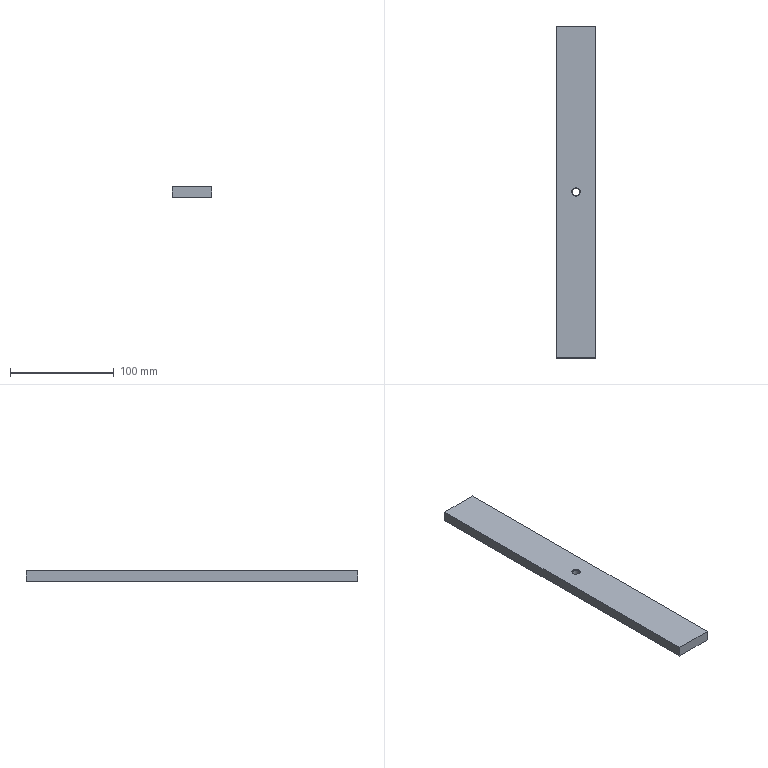Part | STEP file | A14-040 | 1 solid | 10 faces | box 38 x 320 x 10 mm | volume 121232 mm3 | plane 6 | cone 2 | cylinder 2 | commonest cylinder face diameters 6.8 x2
STEP:
#1=CARTESIAN_POINT('',(0.,0.,0.));
#2=DIRECTION('',(0.,0.,1.));
#3=DIRECTION('',(1.,0.,0.));
#4=AXIS2_PLACEMENT_3D('',#1,#2,#3);
#5=CARTESIAN_POINT('',(3.4,0.,4.375));
#6=VERTEX_POINT('',#5);
#7=CARTESIAN_POINT('',(4.025,0.,5.));
#8=VERTEX_POINT('',#7);
#9=CARTESIAN_POINT('',(4.025,0.,5.));
#10=DIRECTION('',(0.7071,0.,0.7071));
#11=VECTOR('',#10,1.);
#12=LINE('',#9,#11);
#13=CARTESIAN_POINT('',(0.,0.,5.));
#14=DIRECTION('',(0.,0.,1.));
#15=DIRECTION('',(1.,0.,0.));
#16=AXIS2_PLACEMENT_3D('',#13,#14,#15);
#17=CONICAL_SURFACE('',#16,4.025,0.7854);
#18=CARTESIAN_POINT('',(6.283,0.));
#19=DIRECTION('',(0.,1.));
#20=VECTOR('',#19,1.);
#21=LINE('',#18,#20);
#22=(GEOMETRIC_REPRESENTATION_CONTEXT(2)PARAMETRIC_REPRESENTATION_CONTEXT()REPRESENTATION_CONTEXT('',''));
#23=DEFINITIONAL_REPRESENTATION('',(#21),#22);
#24=PCURVE('',#17,#23);
#25=CARTESIAN_POINT('',(0.,0.,5.));
#26=DIRECTION('',(0.,0.,1.));
#27=DIRECTION('',(1.,0.,0.));
#28=AXIS2_PLACEMENT_3D('',#25,#26,#27);
#29=CONICAL_SURFACE('',#28,4.025,0.7854);
#30=CARTESIAN_POINT('',(0.,0.));
#31=DIRECTION('',(0.,1.));
#32=VECTOR('',#31,1.);
#33=LINE('',#30,#32);
#34=(GEOMETRIC_REPRESENTATION_CONTEXT(2)PARAMETRIC_REPRESENTATION_CONTEXT()REPRESENTATION_CONTEXT('',''));
#35=DEFINITIONAL_REPRESENTATION('',(#33),#34);
#36=PCURVE('',#29,#35);
#37=SURFACE_CURVE('',#12,(#24,#36),.PCURVE_S1.);
#38=EDGE_CURVE('',#6,#8,#37,.T.);
#39=ORIENTED_EDGE('',*,*,#38,.T.);
#40=CARTESIAN_POINT('',(-4.025,0.,5.));
#41=VERTEX_POINT('',#40);
#42=CARTESIAN_POINT('',(0.,0.,5.));
#43=DIRECTION('',(0.,0.,1.));
#44=DIRECTION('',(1.,0.,0.));
#45=AXIS2_PLACEMENT_3D('',#42,#43,#44);
#46=CIRCLE('',#45,4.025);
#47=CARTESIAN_POINT('',(0.,0.));
#48=DIRECTION('',(1.,0.));
#49=VECTOR('',#48,1.);
#50=LINE('',#47,#49);
#51=(GEOMETRIC_REPRESENTATION_CONTEXT(2)PARAMETRIC_REPRESENTATION_CONTEXT()REPRESENTATION_CONTEXT('',''));
#52=DEFINITIONAL_REPRESENTATION('',(#50),#51);
#53=PCURVE('',#17,#52);
#54=CARTESIAN_POINT('',(0.,0.,5.));
#55=DIRECTION('',(0.,0.,1.));
#56=DIRECTION('',(1.,0.,0.));
#57=AXIS2_PLACEMENT_3D('',#54,#55,#56);
#58=PLANE('',#57);
#59=CARTESIAN_POINT('',(0.,0.));
#60=DIRECTION('',(1.,0.));
#61=AXIS2_PLACEMENT_2D('',#59,#60);
#62=CIRCLE('',#61,4.025);
#63=(GEOMETRIC_REPRESENTATION_CONTEXT(2)PARAMETRIC_REPRESENTATION_CONTEXT()REPRESENTATION_CONTEXT('',''));
#64=DEFINITIONAL_REPRESENTATION('',(#62),#63);
#65=PCURVE('',#58,#64);
#66=SURFACE_CURVE('',#46,(#53,#65),.PCURVE_S1.);
#67=EDGE_CURVE('',#41,#8,#66,.T.);
#68=ORIENTED_EDGE('',*,*,#67,.F.);
#69=CARTESIAN_POINT('',(-3.4,0.,4.375));
#70=VERTEX_POINT('',#69);
#71=CARTESIAN_POINT('',(-4.025,0.,5.));
#72=DIRECTION('',(-0.7071,0.,0.7071));
#73=VECTOR('',#72,1.);
#74=LINE('',#71,#73);
#75=CARTESIAN_POINT('',(3.142,0.));
#76=DIRECTION('',(0.,1.));
#77=VECTOR('',#76,1.);
#78=LINE('',#75,#77);
#79=(GEOMETRIC_REPRESENTATION_CONTEXT(2)PARAMETRIC_REPRESENTATION_CONTEXT()REPRESENTATION_CONTEXT('',''));
#80=DEFINITIONAL_REPRESENTATION('',(#78),#79);
#81=PCURVE('',#17,#80);
#82=CARTESIAN_POINT('',(3.142,0.));
#83=DIRECTION('',(0.,1.));
#84=VECTOR('',#83,1.);
#85=LINE('',#82,#84);
#86=(GEOMETRIC_REPRESENTATION_CONTEXT(2)PARAMETRIC_REPRESENTATION_CONTEXT()REPRESENTATION_CONTEXT('',''));
#87=DEFINITIONAL_REPRESENTATION('',(#85),#86);
#88=PCURVE('',#29,#87);
#89=SURFACE_CURVE('',#74,(#81,#88),.PCURVE_S1.);
#90=EDGE_CURVE('',#70,#41,#89,.T.);
#91=ORIENTED_EDGE('',*,*,#90,.F.);
#92=CARTESIAN_POINT('',(0.,0.,4.375));
#93=DIRECTION('',(0.,0.,1.));
#94=DIRECTION('',(1.,0.,0.));
#95=AXIS2_PLACEMENT_3D('',#92,#93,#94);
#96=CIRCLE('',#95,3.4);
#97=CARTESIAN_POINT('',(0.,-0.625));
#98=DIRECTION('',(1.,0.));
#99=VECTOR('',#98,1.);
#100=LINE('',#97,#99);
#101=(GEOMETRIC_REPRESENTATION_CONTEXT(2)PARAMETRIC_REPRESENTATION_CONTEXT()REPRESENTATION_CONTEXT('',''));
#102=DEFINITIONAL_REPRESENTATION('',(#100),#101);
#103=PCURVE('',#17,#102);
#104=CARTESIAN_POINT('',(0.,0.,5.));
#105=DIRECTION('',(0.,0.,1.));
#106=DIRECTION('',(1.,0.,0.));
#107=AXIS2_PLACEMENT_3D('',#104,#105,#106);
#108=CYLINDRICAL_SURFACE('',#107,3.4);
#109=CARTESIAN_POINT('',(0.,-0.625));
#110=DIRECTION('',(1.,0.));
#111=VECTOR('',#110,1.);
#112=LINE('',#109,#111);
#113=(GEOMETRIC_REPRESENTATION_CONTEXT(2)PARAMETRIC_REPRESENTATION_CONTEXT()REPRESENTATION_CONTEXT('',''));
#114=DEFINITIONAL_REPRESENTATION('',(#112),#113);
#115=PCURVE('',#108,#114);
#116=SURFACE_CURVE('',#96,(#103,#115),.PCURVE_S1.);
#117=EDGE_CURVE('',#70,#6,#116,.T.);
#118=ORIENTED_EDGE('',*,*,#117,.T.);
#119=EDGE_LOOP('',(#39,#68,#91,#118));
#120=FACE_BOUND('',#119,.F.);
#121=ADVANCED_FACE('',(#120),#17,.F.);
#122=CARTESIAN_POINT('',(3.4,0.,-5.));
#123=VERTEX_POINT('',#122);
#124=CARTESIAN_POINT('',(3.4,0.,5.));
#125=DIRECTION('',(0.,0.,1.));
#126=VECTOR('',#125,1.);
#127=LINE('',#124,#126);
#128=CARTESIAN_POINT('',(6.283,0.));
#129=DIRECTION('',(0.,1.));
#130=VECTOR('',#129,1.);
#131=LINE('',#128,#130);
#132=(GEOMETRIC_REPRESENTATION_CONTEXT(2)PARAMETRIC_REPRESENTATION_CONTEXT()REPRESENTATION_CONTEXT('',''));
#133=DEFINITIONAL_REPRESENTATION('',(#131),#132);
#134=PCURVE('',#108,#133);
#135=CARTESIAN_POINT('',(0.,0.,5.));
#136=DIRECTION('',(0.,0.,1.));
#137=DIRECTION('',(1.,0.,0.));
#138=AXIS2_PLACEMENT_3D('',#135,#136,#137);
#139=CYLINDRICAL_SURFACE('',#138,3.4);
#140=CARTESIAN_POINT('',(0.,0.));
#141=DIRECTION('',(0.,1.));
#142=VECTOR('',#141,1.);
#143=LINE('',#140,#142);
#144=(GEOMETRIC_REPRESENTATION_CONTEXT(2)PARAMETRIC_REPRESENTATION_CONTEXT()REPRESENTATION_CONTEXT('',''));
#145=DEFINITIONAL_REPRESENTATION('',(#143),#144);
#146=PCURVE('',#139,#145);
#147=SURFACE_CURVE('',#127,(#134,#146),.PCURVE_S1.);
#148=EDGE_CURVE('',#123,#6,#147,.T.);
#149=ORIENTED_EDGE('',*,*,#148,.T.);
#150=ORIENTED_EDGE('',*,*,#117,.F.);
#151=CARTESIAN_POINT('',(-3.4,0.,-5.));
#152=VERTEX_POINT('',#151);
#153=CARTESIAN_POINT('',(-3.4,0.,5.));
#154=DIRECTION('',(0.,0.,1.));
#155=VECTOR('',#154,1.);
#156=LINE('',#153,#155);
#157=CARTESIAN_POINT('',(3.142,0.));
#158=DIRECTION('',(0.,1.));
#159=VECTOR('',#158,1.);
#160=LINE('',#157,#159);
#161=(GEOMETRIC_REPRESENTATION_CONTEXT(2)PARAMETRIC_REPRESENTATION_CONTEXT()REPRESENTATION_CONTEXT('',''));
#162=DEFINITIONAL_REPRESENTATION('',(#160),#161);
#163=PCURVE('',#108,#162);
#164=CARTESIAN_POINT('',(3.142,0.));
#165=DIRECTION('',(0.,1.));
#166=VECTOR('',#165,1.);
#167=LINE('',#164,#166);
#168=(GEOMETRIC_REPRESENTATION_CONTEXT(2)PARAMETRIC_REPRESENTATION_CONTEXT()REPRESENTATION_CONTEXT('',''));
#169=DEFINITIONAL_REPRESENTATION('',(#167),#168);
#170=PCURVE('',#139,#169);
#171=SURFACE_CURVE('',#156,(#163,#170),.PCURVE_S1.);
#172=EDGE_CURVE('',#152,#70,#171,.T.);
#173=ORIENTED_EDGE('',*,*,#172,.F.);
#174=CARTESIAN_POINT('',(0.,0.,-5.));
#175=DIRECTION('',(0.,0.,1.));
#176=DIRECTION('',(1.,0.,0.));
#177=AXIS2_PLACEMENT_3D('',#174,#175,#176);
#178=CIRCLE('',#177,3.4);
#179=CARTESIAN_POINT('',(0.,-10.));
#180=DIRECTION('',(1.,0.));
#181=VECTOR('',#180,1.);
#182=LINE('',#179,#181);
#183=(GEOMETRIC_REPRESENTATION_CONTEXT(2)PARAMETRIC_REPRESENTATION_CONTEXT()REPRESENTATION_CONTEXT('',''));
#184=DEFINITIONAL_REPRESENTATION('',(#182),#183);
#185=PCURVE('',#108,#184);
#186=CARTESIAN_POINT('',(0.,0.,-5.));
#187=DIRECTION('',(0.,0.,1.));
#188=DIRECTION('',(1.,0.,0.));
#189=AXIS2_PLACEMENT_3D('',#186,#187,#188);
#190=PLANE('',#189);
#191=CARTESIAN_POINT('',(0.,0.));
#192=DIRECTION('',(1.,0.));
#193=AXIS2_PLACEMENT_2D('',#191,#192);
#194=CIRCLE('',#193,3.4);
#195=(GEOMETRIC_REPRESENTATION_CONTEXT(2)PARAMETRIC_REPRESENTATION_CONTEXT()REPRESENTATION_CONTEXT('',''));
#196=DEFINITIONAL_REPRESENTATION('',(#194),#195);
#197=PCURVE('',#190,#196);
#198=SURFACE_CURVE('',#178,(#185,#197),.PCURVE_S1.);
#199=EDGE_CURVE('',#152,#123,#198,.T.);
#200=ORIENTED_EDGE('',*,*,#199,.T.);
#201=EDGE_LOOP('',(#149,#150,#173,#200));
#202=FACE_BOUND('',#201,.F.);
#203=ADVANCED_FACE('',(#202),#108,.F.);
#204=CARTESIAN_POINT('',(19.,-160.,-5.));
#205=VERTEX_POINT('',#204);
#206=CARTESIAN_POINT('',(19.,160.,-5.));
#207=VERTEX_POINT('',#206);
#208=CARTESIAN_POINT('',(19.,160.,-5.));
#209=DIRECTION('',(0.,1.,0.));
#210=VECTOR('',#209,1.);
#211=LINE('',#208,#210);
#212=CARTESIAN_POINT('',(19.,160.,5.));
#213=DIRECTION('',(-1.,0.,0.));
#214=DIRECTION('',(0.,0.,1.));
#215=AXIS2_PLACEMENT_3D('',#212,#213,#214);
#216=PLANE('',#215);
#217=CARTESIAN_POINT('',(-10.,0.));
#218=DIRECTION('',(0.,1.));
#219=VECTOR('',#218,1.);
#220=LINE('',#217,#219);
#221=(GEOMETRIC_REPRESENTATION_CONTEXT(2)PARAMETRIC_REPRESENTATION_CONTEXT()REPRESENTATION_CONTEXT('',''));
#222=DEFINITIONAL_REPRESENTATION('',(#220),#221);
#223=PCURVE('',#216,#222);
#224=CARTESIAN_POINT('',(19.,160.));
#225=DIRECTION('',(0.,1.));
#226=VECTOR('',#225,1.);
#227=LINE('',#224,#226);
#228=(GEOMETRIC_REPRESENTATION_CONTEXT(2)PARAMETRIC_REPRESENTATION_CONTEXT()REPRESENTATION_CONTEXT('',''));
#229=DEFINITIONAL_REPRESENTATION('',(#227),#228);
#230=PCURVE('',#190,#229);
#231=SURFACE_CURVE('',#211,(#223,#230),.PCURVE_S1.);
#232=EDGE_CURVE('',#205,#207,#231,.T.);
#233=ORIENTED_EDGE('',*,*,#232,.T.);
#234=CARTESIAN_POINT('',(19.,160.,5.));
#235=VERTEX_POINT('',#234);
#236=CARTESIAN_POINT('',(19.,160.,5.));
#237=DIRECTION('',(0.,0.,-1.));
#238=VECTOR('',#237,1.);
#239=LINE('',#236,#238);
#240=CARTESIAN_POINT('',(0.,0.));
#241=DIRECTION('',(-1.,0.));
#242=VECTOR('',#241,1.);
#243=LINE('',#240,#242);
#244=(GEOMETRIC_REPRESENTATION_CONTEXT(2)PARAMETRIC_REPRESENTATION_CONTEXT()REPRESENTATION_CONTEXT('',''));
#245=DEFINITIONAL_REPRESENTATION('',(#243),#244);
#246=PCURVE('',#216,#245);
#247=CARTESIAN_POINT('',(-19.,160.,5.));
#248=DIRECTION('',(0.,-1.,0.));
#249=DIRECTION('',(0.,0.,-1.));
#250=AXIS2_PLACEMENT_3D('',#247,#248,#249);
#251=PLANE('',#250);
#252=CARTESIAN_POINT('',(0.,38.));
#253=DIRECTION('',(1.,0.));
#254=VECTOR('',#253,1.);
#255=LINE('',#252,#254);
#256=(GEOMETRIC_REPRESENTATION_CONTEXT(2)PARAMETRIC_REPRESENTATION_CONTEXT()REPRESENTATION_CONTEXT('',''));
#257=DEFINITIONAL_REPRESENTATION('',(#255),#256);
#258=PCURVE('',#251,#257);
#259=SURFACE_CURVE('',#239,(#246,#258),.PCURVE_S1.);
#260=EDGE_CURVE('',#235,#207,#259,.T.);
#261=ORIENTED_EDGE('',*,*,#260,.F.);
#262=CARTESIAN_POINT('',(19.,-160.,5.));
#263=VERTEX_POINT('',#262);
#264=CARTESIAN_POINT('',(19.,160.,5.));
#265=DIRECTION('',(0.,1.,0.));
#266=VECTOR('',#265,1.);
#267=LINE('',#264,#266);
#268=CARTESIAN_POINT('',(0.,0.));
#269=DIRECTION('',(0.,1.));
#270=VECTOR('',#269,1.);
#271=LINE('',#268,#270);
#272=(GEOMETRIC_REPRESENTATION_CONTEXT(2)PARAMETRIC_REPRESENTATION_CONTEXT()REPRESENTATION_CONTEXT('',''));
#273=DEFINITIONAL_REPRESENTATION('',(#271),#272);
#274=PCURVE('',#216,#273);
#275=CARTESIAN_POINT('',(19.,160.));
#276=DIRECTION('',(0.,1.));
#277=VECTOR('',#276,1.);
#278=LINE('',#275,#277);
#279=(GEOMETRIC_REPRESENTATION_CONTEXT(2)PARAMETRIC_REPRESENTATION_CONTEXT()REPRESENTATION_CONTEXT('',''));
#280=DEFINITIONAL_REPRESENTATION('',(#278),#279);
#281=PCURVE('',#58,#280);
#282=SURFACE_CURVE('',#267,(#274,#281),.PCURVE_S1.);
#283=EDGE_CURVE('',#263,#235,#282,.T.);
#284=ORIENTED_EDGE('',*,*,#283,.F.);
#285=CARTESIAN_POINT('',(19.,-160.,5.));
#286=DIRECTION('',(0.,0.,-1.));
#287=VECTOR('',#286,1.);
#288=LINE('',#285,#287);
#289=CARTESIAN_POINT('',(0.,-320.));
#290=DIRECTION('',(-1.,0.));
#291=VECTOR('',#290,1.);
#292=LINE('',#289,#291);
#293=(GEOMETRIC_REPRESENTATION_CONTEXT(2)PARAMETRIC_REPRESENTATION_CONTEXT()REPRESENTATION_CONTEXT('',''));
#294=DEFINITIONAL_REPRESENTATION('',(#292),#293);
#295=PCURVE('',#216,#294);
#296=CARTESIAN_POINT('',(-19.,-160.,5.));
#297=DIRECTION('',(0.,1.,0.));
#298=DIRECTION('',(0.,0.,1.));
#299=AXIS2_PLACEMENT_3D('',#296,#297,#298);
#300=PLANE('',#299);
#301=CARTESIAN_POINT('',(0.,38.));
#302=DIRECTION('',(-1.,0.));
#303=VECTOR('',#302,1.);
#304=LINE('',#301,#303);
#305=(GEOMETRIC_REPRESENTATION_CONTEXT(2)PARAMETRIC_REPRESENTATION_CONTEXT()REPRESENTATION_CONTEXT('',''));
#306=DEFINITIONAL_REPRESENTATION('',(#304),#305);
#307=PCURVE('',#300,#306);
#308=SURFACE_CURVE('',#288,(#295,#307),.PCURVE_S1.);
#309=EDGE_CURVE('',#263,#205,#308,.T.);
#310=ORIENTED_EDGE('',*,*,#309,.T.);
#311=EDGE_LOOP('',(#233,#261,#284,#310));
#312=FACE_BOUND('',#311,.T.);
#313=ADVANCED_FACE('',(#312),#216,.F.);
#314=CARTESIAN_POINT('',(-19.,160.,-5.));
#315=VERTEX_POINT('',#314);
#316=CARTESIAN_POINT('',(-19.,160.,-5.));
#317=DIRECTION('',(-1.,0.,0.));
#318=VECTOR('',#317,1.);
#319=LINE('',#316,#318);
#320=CARTESIAN_POINT('',(10.,0.));
#321=DIRECTION('',(0.,-1.));
#322=VECTOR('',#321,1.);
#323=LINE('',#320,#322);
#324=(GEOMETRIC_REPRESENTATION_CONTEXT(2)PARAMETRIC_REPRESENTATION_CONTEXT()REPRESENTATION_CONTEXT('',''));
#325=DEFINITIONAL_REPRESENTATION('',(#323),#324);
#326=PCURVE('',#251,#325);
#327=CARTESIAN_POINT('',(-19.,160.));
#328=DIRECTION('',(-1.,0.));
#329=VECTOR('',#328,1.);
#330=LINE('',#327,#329);
#331=(GEOMETRIC_REPRESENTATION_CONTEXT(2)PARAMETRIC_REPRESENTATION_CONTEXT()REPRESENTATION_CONTEXT('',''));
#332=DEFINITIONAL_REPRESENTATION('',(#330),#331);
#333=PCURVE('',#190,#332);
#334=SURFACE_CURVE('',#319,(#326,#333),.PCURVE_S1.);
#335=EDGE_CURVE('',#207,#315,#334,.T.);
#336=ORIENTED_EDGE('',*,*,#335,.T.);
#337=CARTESIAN_POINT('',(-19.,160.,5.));
#338=VERTEX_POINT('',#337);
#339=CARTESIAN_POINT('',(-19.,160.,5.));
#340=DIRECTION('',(0.,0.,-1.));
#341=VECTOR('',#340,1.);
#342=LINE('',#339,#341);
#343=CARTESIAN_POINT('',(0.,0.));
#344=DIRECTION('',(1.,0.));
#345=VECTOR('',#344,1.);
#346=LINE('',#343,#345);
#347=(GEOMETRIC_REPRESENTATION_CONTEXT(2)PARAMETRIC_REPRESENTATION_CONTEXT()REPRESENTATION_CONTEXT('',''));
#348=DEFINITIONAL_REPRESENTATION('',(#346),#347);
#349=PCURVE('',#251,#348);
#350=CARTESIAN_POINT('',(-19.,160.,5.));
#351=DIRECTION('',(1.,0.,0.));
#352=DIRECTION('',(0.,0.,-1.));
#353=AXIS2_PLACEMENT_3D('',#350,#351,#352);
#354=PLANE('',#353);
#355=CARTESIAN_POINT('',(0.,0.));
#356=DIRECTION('',(1.,0.));
#357=VECTOR('',#356,1.);
#358=LINE('',#355,#357);
#359=(GEOMETRIC_REPRESENTATION_CONTEXT(2)PARAMETRIC_REPRESENTATION_CONTEXT()REPRESENTATION_CONTEXT('',''));
#360=DEFINITIONAL_REPRESENTATION('',(#358),#359);
#361=PCURVE('',#354,#360);
#362=SURFACE_CURVE('',#342,(#349,#361),.PCURVE_S1.);
#363=EDGE_CURVE('',#338,#315,#362,.T.);
#364=ORIENTED_EDGE('',*,*,#363,.F.);
#365=CARTESIAN_POINT('',(-19.,160.,5.));
#366=DIRECTION('',(-1.,0.,0.));
#367=VECTOR('',#366,1.);
#368=LINE('',#365,#367);
#369=CARTESIAN_POINT('',(0.,0.));
#370=DIRECTION('',(0.,-1.));
#371=VECTOR('',#370,1.);
#372=LINE('',#369,#371);
#373=(GEOMETRIC_REPRESENTATION_CONTEXT(2)PARAMETRIC_REPRESENTATION_CONTEXT()REPRESENTATION_CONTEXT('',''));
#374=DEFINITIONAL_REPRESENTATION('',(#372),#373);
#375=PCURVE('',#251,#374);
#376=CARTESIAN_POINT('',(-19.,160.));
#377=DIRECTION('',(-1.,0.));
#378=VECTOR('',#377,1.);
#379=LINE('',#376,#378);
#380=(GEOMETRIC_REPRESENTATION_CONTEXT(2)PARAMETRIC_REPRESENTATION_CONTEXT()REPRESENTATION_CONTEXT('',''));
#381=DEFINITIONAL_REPRESENTATION('',(#379),#380);
#382=PCURVE('',#58,#381);
#383=SURFACE_CURVE('',#368,(#375,#382),.PCURVE_S1.);
#384=EDGE_CURVE('',#235,#338,#383,.T.);
#385=ORIENTED_EDGE('',*,*,#384,.F.);
#386=ORIENTED_EDGE('',*,*,#260,.T.);
#387=EDGE_LOOP('',(#336,#364,#385,#386));
#388=FACE_BOUND('',#387,.T.);
#389=ADVANCED_FACE('',(#388),#251,.F.);
#390=CARTESIAN_POINT('',(-19.,-160.,-5.));
#391=VERTEX_POINT('',#390);
#392=CARTESIAN_POINT('',(-19.,160.,-5.));
#393=DIRECTION('',(0.,-1.,0.));
#394=VECTOR('',#393,1.);
#395=LINE('',#392,#394);
#396=CARTESIAN_POINT('',(10.,0.));
#397=DIRECTION('',(0.,-1.));
#398=VECTOR('',#397,1.);
#399=LINE('',#396,#398);
#400=(GEOMETRIC_REPRESENTATION_CONTEXT(2)PARAMETRIC_REPRESENTATION_CONTEXT()REPRESENTATION_CONTEXT('',''));
#401=DEFINITIONAL_REPRESENTATION('',(#399),#400);
#402=PCURVE('',#354,#401);
#403=CARTESIAN_POINT('',(-19.,160.));
#404=DIRECTION('',(0.,-1.));
#405=VECTOR('',#404,1.);
#406=LINE('',#403,#405);
#407=(GEOMETRIC_REPRESENTATION_CONTEXT(2)PARAMETRIC_REPRESENTATION_CONTEXT()REPRESENTATION_CONTEXT('',''));
#408=DEFINITIONAL_REPRESENTATION('',(#406),#407);
#409=PCURVE('',#190,#408);
#410=SURFACE_CURVE('',#395,(#402,#409),.PCURVE_S1.);
#411=EDGE_CURVE('',#315,#391,#410,.T.);
#412=ORIENTED_EDGE('',*,*,#411,.T.);
#413=CARTESIAN_POINT('',(-19.,-160.,5.));
#414=VERTEX_POINT('',#413);
#415=CARTESIAN_POINT('',(-19.,-160.,5.));
#416=DIRECTION('',(0.,0.,-1.));
#417=VECTOR('',#416,1.);
#418=LINE('',#415,#417);
#419=CARTESIAN_POINT('',(0.,-320.));
#420=DIRECTION('',(1.,0.));
#421=VECTOR('',#420,1.);
#422=LINE('',#419,#421);
#423=(GEOMETRIC_REPRESENTATION_CONTEXT(2)PARAMETRIC_REPRESENTATION_CONTEXT()REPRESENTATION_CONTEXT('',''));
#424=DEFINITIONAL_REPRESENTATION('',(#422),#423);
#425=PCURVE('',#354,#424);
#426=CARTESIAN_POINT('',(0.,0.));
#427=DIRECTION('',(-1.,0.));
#428=VECTOR('',#427,1.);
#429=LINE('',#426,#428);
#430=(GEOMETRIC_REPRESENTATION_CONTEXT(2)PARAMETRIC_REPRESENTATION_CONTEXT()REPRESENTATION_CONTEXT('',''));
#431=DEFINITIONAL_REPRESENTATION('',(#429),#430);
#432=PCURVE('',#300,#431);
#433=SURFACE_CURVE('',#418,(#425,#432),.PCURVE_S1.);
#434=EDGE_CURVE('',#414,#391,#433,.T.);
#435=ORIENTED_EDGE('',*,*,#434,.F.);
#436=CARTESIAN_POINT('',(-19.,160.,5.));
#437=DIRECTION('',(0.,-1.,0.));
#438=VECTOR('',#437,1.);
#439=LINE('',#436,#438);
#440=CARTESIAN_POINT('',(0.,0.));
#441=DIRECTION('',(0.,-1.));
#442=VECTOR('',#441,1.);
#443=LINE('',#440,#442);
#444=(GEOMETRIC_REPRESENTATION_CONTEXT(2)PARAMETRIC_REPRESENTATION_CONTEXT()REPRESENTATION_CONTEXT('',''));
#445=DEFINITIONAL_REPRESENTATION('',(#443),#444);
#446=PCURVE('',#354,#445);
#447=CARTESIAN_POINT('',(-19.,160.));
#448=DIRECTION('',(0.,-1.));
#449=VECTOR('',#448,1.);
#450=LINE('',#447,#449);
#451=(GEOMETRIC_REPRESENTATION_CONTEXT(2)PARAMETRIC_REPRESENTATION_CONTEXT()REPRESENTATION_CONTEXT('',''));
#452=DEFINITIONAL_REPRESENTATION('',(#450),#451);
#453=PCURVE('',#58,#452);
#454=SURFACE_CURVE('',#439,(#446,#453),.PCURVE_S1.);
#455=EDGE_CURVE('',#338,#414,#454,.T.);
#456=ORIENTED_EDGE('',*,*,#455,.F.);
#457=ORIENTED_EDGE('',*,*,#363,.T.);
#458=EDGE_LOOP('',(#412,#435,#456,#457));
#459=FACE_BOUND('',#458,.T.);
#460=ADVANCED_FACE('',(#459),#354,.F.);
#461=CARTESIAN_POINT('',(-19.,-160.,-5.));
#462=DIRECTION('',(1.,0.,0.));
#463=VECTOR('',#462,1.);
#464=LINE('',#461,#463);
#465=CARTESIAN_POINT('',(-10.,0.));
#466=DIRECTION('',(0.,1.));
#467=VECTOR('',#466,1.);
#468=LINE('',#465,#467);
#469=(GEOMETRIC_REPRESENTATION_CONTEXT(2)PARAMETRIC_REPRESENTATION_CONTEXT()REPRESENTATION_CONTEXT('',''));
#470=DEFINITIONAL_REPRESENTATION('',(#468),#469);
#471=PCURVE('',#300,#470);
#472=CARTESIAN_POINT('',(-19.,-160.));
#473=DIRECTION('',(1.,0.));
#474=VECTOR('',#473,1.);
#475=LINE('',#472,#474);
#476=(GEOMETRIC_REPRESENTATION_CONTEXT(2)PARAMETRIC_REPRESENTATION_CONTEXT()REPRESENTATION_CONTEXT('',''));
#477=DEFINITIONAL_REPRESENTATION('',(#475),#476);
#478=PCURVE('',#190,#477);
#479=SURFACE_CURVE('',#464,(#471,#478),.PCURVE_S1.);
#480=EDGE_CURVE('',#391,#205,#479,.T.);
#481=ORIENTED_EDGE('',*,*,#480,.T.);
#482=ORIENTED_EDGE('',*,*,#309,.F.);
#483=CARTESIAN_POINT('',(-19.,-160.,5.));
#484=DIRECTION('',(1.,0.,0.));
#485=VECTOR('',#484,1.);
#486=LINE('',#483,#485);
#487=CARTESIAN_POINT('',(0.,0.));
#488=DIRECTION('',(0.,1.));
#489=VECTOR('',#488,1.);
#490=LINE('',#487,#489);
#491=(GEOMETRIC_REPRESENTATION_CONTEXT(2)PARAMETRIC_REPRESENTATION_CONTEXT()REPRESENTATION_CONTEXT('',''));
#492=DEFINITIONAL_REPRESENTATION('',(#490),#491);
#493=PCURVE('',#300,#492);
#494=CARTESIAN_POINT('',(-19.,-160.));
#495=DIRECTION('',(1.,0.));
#496=VECTOR('',#495,1.);
#497=LINE('',#494,#496);
#498=(GEOMETRIC_REPRESENTATION_CONTEXT(2)PARAMETRIC_REPRESENTATION_CONTEXT()REPRESENTATION_CONTEXT('',''));
#499=DEFINITIONAL_REPRESENTATION('',(#497),#498);
#500=PCURVE('',#58,#499);
#501=SURFACE_CURVE('',#486,(#493,#500),.PCURVE_S1.);
#502=EDGE_CURVE('',#414,#263,#501,.T.);
#503=ORIENTED_EDGE('',*,*,#502,.F.);
#504=ORIENTED_EDGE('',*,*,#434,.T.);
#505=EDGE_LOOP('',(#481,#482,#503,#504));
#506=FACE_BOUND('',#505,.T.);
#507=ADVANCED_FACE('',(#506),#300,.F.);
#508=CARTESIAN_POINT('',(0.,0.,5.));
#509=DIRECTION('',(0.,0.,1.));
#510=DIRECTION('',(1.,0.,0.));
#511=AXIS2_PLACEMENT_3D('',#508,#509,#510);
#512=CIRCLE('',#511,4.025);
#513=CARTESIAN_POINT('',(0.,0.));
#514=DIRECTION('',(1.,0.));
#515=AXIS2_PLACEMENT_2D('',#513,#514);
#516=CIRCLE('',#515,4.025);
#517=(GEOMETRIC_REPRESENTATION_CONTEXT(2)PARAMETRIC_REPRESENTATION_CONTEXT()REPRESENTATION_CONTEXT('',''));
#518=DEFINITIONAL_REPRESENTATION('',(#516),#517);
#519=PCURVE('',#58,#518);
#520=CARTESIAN_POINT('',(0.,0.));
#521=DIRECTION('',(1.,0.));
#522=VECTOR('',#521,1.);
#523=LINE('',#520,#522);
#524=(GEOMETRIC_REPRESENTATION_CONTEXT(2)PARAMETRIC_REPRESENTATION_CONTEXT()REPRESENTATION_CONTEXT('',''));
#525=DEFINITIONAL_REPRESENTATION('',(#523),#524);
#526=PCURVE('',#29,#525);
#527=SURFACE_CURVE('',#512,(#519,#526),.PCURVE_S1.);
#528=EDGE_CURVE('',#8,#41,#527,.T.);
#529=ORIENTED_EDGE('',*,*,#528,.F.);
#530=ORIENTED_EDGE('',*,*,#67,.F.);
#531=EDGE_LOOP('',(#529,#530));
#532=FACE_BOUND('',#531,.T.);
#533=ORIENTED_EDGE('',*,*,#283,.T.);
#534=ORIENTED_EDGE('',*,*,#384,.T.);
#535=ORIENTED_EDGE('',*,*,#455,.T.);
#536=ORIENTED_EDGE('',*,*,#502,.T.);
#537=EDGE_LOOP('',(#533,#534,#535,#536));
#538=FACE_BOUND('',#537,.T.);
#539=ADVANCED_FACE('',(#532,#538),#58,.T.);
#540=CARTESIAN_POINT('',(0.,0.,-5.));
#541=DIRECTION('',(0.,0.,1.));
#542=DIRECTION('',(1.,0.,0.));
#543=AXIS2_PLACEMENT_3D('',#540,#541,#542);
#544=CIRCLE('',#543,3.4);
#545=CARTESIAN_POINT('',(0.,0.));
#546=DIRECTION('',(1.,0.));
#547=AXIS2_PLACEMENT_2D('',#545,#546);
#548=CIRCLE('',#547,3.4);
#549=(GEOMETRIC_REPRESENTATION_CONTEXT(2)PARAMETRIC_REPRESENTATION_CONTEXT()REPRESENTATION_CONTEXT('',''));
#550=DEFINITIONAL_REPRESENTATION('',(#548),#549);
#551=PCURVE('',#190,#550);
#552=CARTESIAN_POINT('',(0.,-10.));
#553=DIRECTION('',(1.,0.));
#554=VECTOR('',#553,1.);
#555=LINE('',#552,#554);
#556=(GEOMETRIC_REPRESENTATION_CONTEXT(2)PARAMETRIC_REPRESENTATION_CONTEXT()REPRESENTATION_CONTEXT('',''));
#557=DEFINITIONAL_REPRESENTATION('',(#555),#556);
#558=PCURVE('',#139,#557);
#559=SURFACE_CURVE('',#544,(#551,#558),.PCURVE_S1.);
#560=EDGE_CURVE('',#123,#152,#559,.T.);
#561=ORIENTED_EDGE('',*,*,#560,.T.);
#562=ORIENTED_EDGE('',*,*,#199,.T.);
#563=EDGE_LOOP('',(#561,#562));
#564=FACE_BOUND('',#563,.T.);
#565=ORIENTED_EDGE('',*,*,#232,.F.);
#566=ORIENTED_EDGE('',*,*,#480,.F.);
#567=ORIENTED_EDGE('',*,*,#411,.F.);
#568=ORIENTED_EDGE('',*,*,#335,.F.);
#569=EDGE_LOOP('',(#565,#566,#567,#568));
#570=FACE_BOUND('',#569,.T.);
#571=ADVANCED_FACE('',(#564,#570),#190,.F.);
#572=CARTESIAN_POINT('',(0.,0.,4.375));
#573=DIRECTION('',(0.,0.,1.));
#574=DIRECTION('',(1.,0.,0.));
#575=AXIS2_PLACEMENT_3D('',#572,#573,#574);
#576=CIRCLE('',#575,3.4);
#577=CARTESIAN_POINT('',(0.,-0.625));
#578=DIRECTION('',(1.,0.));
#579=VECTOR('',#578,1.);
#580=LINE('',#577,#579);
#581=(GEOMETRIC_REPRESENTATION_CONTEXT(2)PARAMETRIC_REPRESENTATION_CONTEXT()REPRESENTATION_CONTEXT('',''));
#582=DEFINITIONAL_REPRESENTATION('',(#580),#581);
#583=PCURVE('',#139,#582);
#584=CARTESIAN_POINT('',(0.,-0.625));
#585=DIRECTION('',(1.,0.));
#586=VECTOR('',#585,1.);
#587=LINE('',#584,#586);
#588=(GEOMETRIC_REPRESENTATION_CONTEXT(2)PARAMETRIC_REPRESENTATION_CONTEXT()REPRESENTATION_CONTEXT('',''));
#589=DEFINITIONAL_REPRESENTATION('',(#587),#588);
#590=PCURVE('',#29,#589);
#591=SURFACE_CURVE('',#576,(#583,#590),.PCURVE_S1.);
#592=EDGE_CURVE('',#6,#70,#591,.T.);
#593=ORIENTED_EDGE('',*,*,#592,.F.);
#594=ORIENTED_EDGE('',*,*,#148,.F.);
#595=ORIENTED_EDGE('',*,*,#560,.T.);
#596=ORIENTED_EDGE('',*,*,#172,.T.);
#597=EDGE_LOOP('',(#593,#594,#595,#596));
#598=FACE_BOUND('',#597,.F.);
#599=ADVANCED_FACE('',(#598),#139,.F.);
#600=ORIENTED_EDGE('',*,*,#528,.F.);
#601=ORIENTED_EDGE('',*,*,#38,.F.);
#602=ORIENTED_EDGE('',*,*,#592,.T.);
#603=ORIENTED_EDGE('',*,*,#90,.T.);
#604=EDGE_LOOP('',(#600,#601,#602,#603));
#605=FACE_BOUND('',#604,.F.);
#606=ADVANCED_FACE('',(#605),#29,.F.);
#607=CLOSED_SHELL('',(#121,#203,#313,#389,#460,#507,#539,#571,#599,#606));
#608=MANIFOLD_SOLID_BREP('',#607);
#609=(LENGTH_UNIT()NAMED_UNIT(*)SI_UNIT(.MILLI.,.METRE.));
#610=UNCERTAINTY_MEASURE_WITH_UNIT(LENGTH_MEASURE(0.0000001),#609,'','');
#611=(NAMED_UNIT(*)PLANE_ANGLE_UNIT()SI_UNIT($,.RADIAN.));
#612=(NAMED_UNIT(*)SI_UNIT($,.STERADIAN.)SOLID_ANGLE_UNIT());
#613=(GEOMETRIC_REPRESENTATION_CONTEXT(3)GLOBAL_UNCERTAINTY_ASSIGNED_CONTEXT((#610))GLOBAL_UNIT_ASSIGNED_CONTEXT((#609,#611,#612))REPRESENTATION_CONTEXT('',''));
#614=ADVANCED_BREP_SHAPE_REPRESENTATION('',(#4,#608),#613);